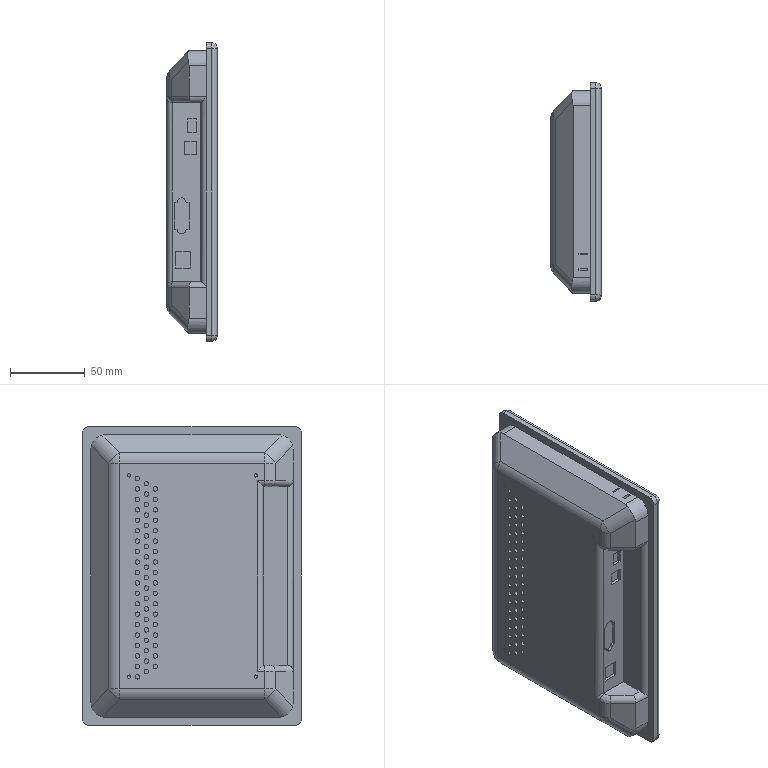Part | STEP file | MT6070iH5[MT6070iH5]_MT6070iH5 | 1 solid | 299 faces | box 34 x 146.5 x 200.4 mm | volume 782719 mm3 | cylinder 154 | plane 127 | spline 10 | cone 8 | commonest cylinder face diameters 3 x114 8 x16 20 x13 2.261 x8 6 x3